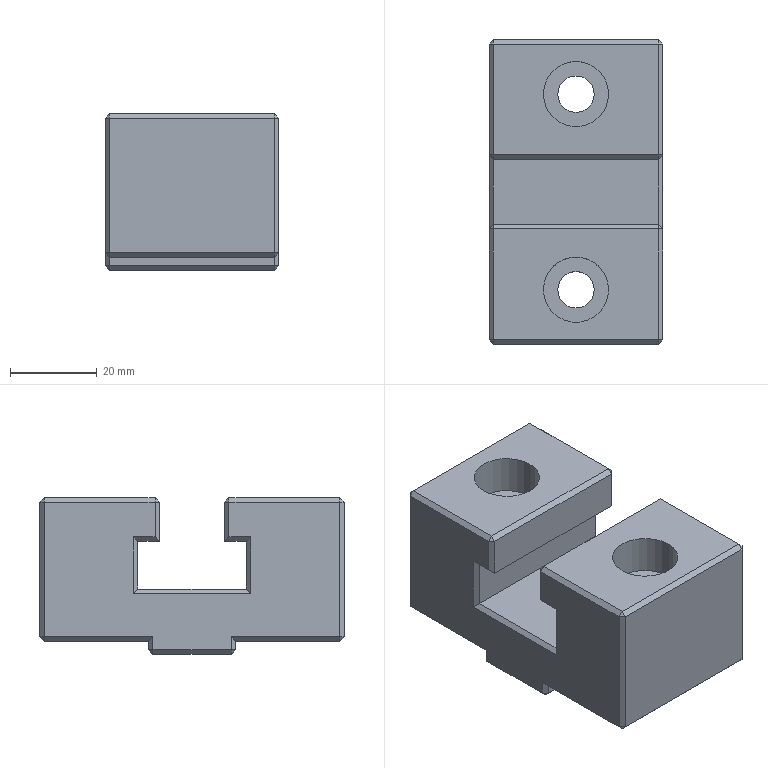Part | STEP file | BATENTE PLACA EXTRATORA - Torre - 1 cav | 1 solid | 84 faces | box 40 x 70 x 36 mm | volume 71533 mm3 | plane 76 | cylinder 8 | commonest cylinder face diameters 8.4 x4 15 x4